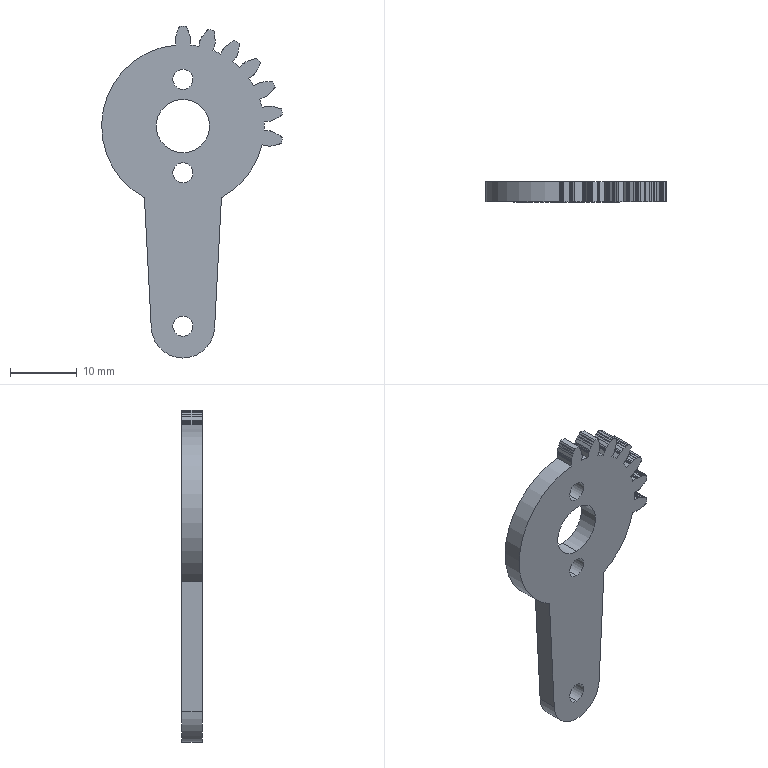Part | STEP file | Claw gear_1 | 1 solid | 253 faces | box 27.091 x 3 x 49.757 mm | volume 1979 mm3 | plane 186 | cylinder 67 | commonest cylinder face diameters 5.449 x14 17.652 x14 33.818 x14 24.375 x8 30 x7 3 x6